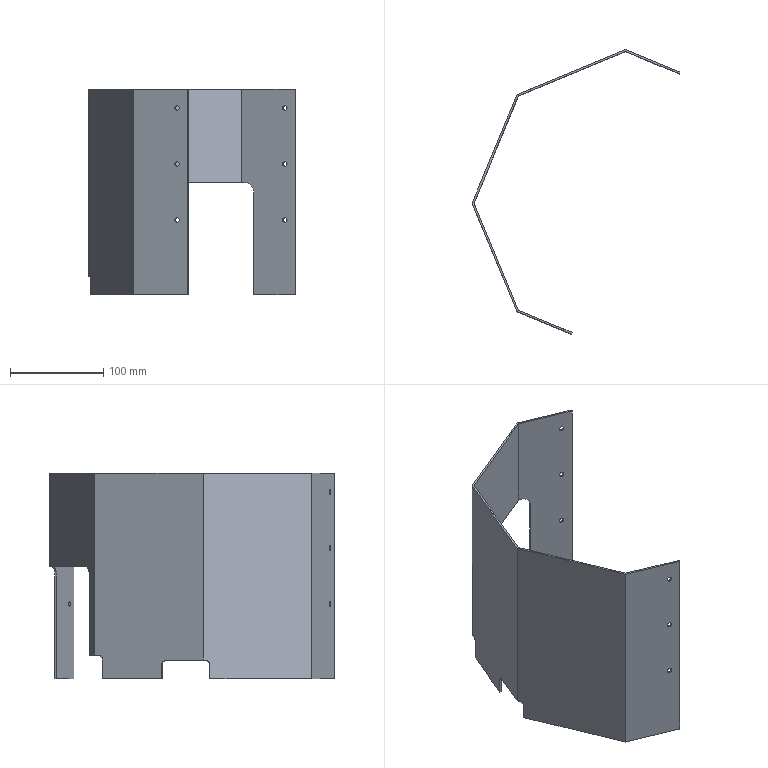Part | SolidWorks | features ICE 6, Fillet 3, Cut 2, Extrusion 1, RefAxis 1, Shell 1 | 1 solid | 41 faces | box 222.691 x 304.953 x 220 mm | volume 186706 mm3 | plane 24 | cylinder 17 | commonest cylinder face diameters 5 x12 10 x3 20 x2
STEP:
#1=CARTESIAN_POINT('',(-66.179,-134.946,80.));
#2=VERTEX_POINT('',#1);
#3=CARTESIAN_POINT('',(-70.799,-133.033,80.));
#4=VERTEX_POINT('',#3);
#5=CARTESIAN_POINT('',(-68.489,-133.99,80.));
#6=DIRECTION('',(0.3827,0.9239,0.));
#7=DIRECTION('',(-0.9239,0.3827,0.));
#8=AXIS2_PLACEMENT_3D('',#5,#6,#7);
#9=CIRCLE('',#8,2.5);
#10=EDGE_CURVE('',#2,#4,#9,.T.);
#11=ORIENTED_EDGE('',*,*,#10,.T.);
#12=CARTESIAN_POINT('',(-71.564,-134.881,80.));
#13=VERTEX_POINT('',#12);
#14=CARTESIAN_POINT('',(53.29,166.544,80.));
#15=DIRECTION('',(-0.3827,-0.9239,0.));
#16=VECTOR('',#15,1000.);
#17=LINE('',#14,#16);
#18=EDGE_CURVE('',#4,#13,#17,.T.);
#19=ORIENTED_EDGE('',*,*,#18,.T.);
#20=CARTESIAN_POINT('',(-66.945,-136.794,80.));
#21=VERTEX_POINT('',#20);
#22=CARTESIAN_POINT('',(-69.254,-135.837,80.));
#23=DIRECTION('',(-0.3827,-0.9239,0.));
#24=DIRECTION('',(0.9239,-0.3827,0.));
#25=AXIS2_PLACEMENT_3D('',#22,#23,#24);
#26=CIRCLE('',#25,2.5);
#27=EDGE_CURVE('',#13,#21,#26,.T.);
#28=ORIENTED_EDGE('',*,*,#27,.T.);
#29=CARTESIAN_POINT('',(57.91,164.631,80.));
#30=DIRECTION('',(-0.3827,-0.9239,0.));
#31=VECTOR('',#30,1000.);
#32=LINE('',#29,#31);
#33=EDGE_CURVE('',#2,#21,#32,.T.);
#34=ORIENTED_EDGE('',*,*,#33,.F.);
#35=EDGE_LOOP('',(#11,#19,#28,#34));
#36=FACE_OUTER_BOUND('',#35,.T.);
#37=CARTESIAN_POINT('',(55.6,165.587,80.));
#38=DIRECTION('',(-0.3827,-0.9239,0.));
#39=DIRECTION('',(0.9239,-0.3827,0.));
#40=AXIS2_PLACEMENT_3D('',#37,#38,#39);
#41=CYLINDRICAL_SURFACE('',#40,2.5);
#42=ADVANCED_FACE('',(#36),#41,.F.);
#43=CARTESIAN_POINT('',(44.772,145.979,80.));
#44=VERTEX_POINT('',#43);
#45=CARTESIAN_POINT('',(49.391,144.065,80.));
#46=VERTEX_POINT('',#45);
#47=CARTESIAN_POINT('',(47.081,145.022,80.));
#48=DIRECTION('',(-0.3827,-0.9239,0.));
#49=DIRECTION('',(0.9239,-0.3827,0.));
#50=AXIS2_PLACEMENT_3D('',#47,#48,#49);
#51=CIRCLE('',#50,2.5);
#52=EDGE_CURVE('',#44,#46,#51,.T.);
#53=ORIENTED_EDGE('',*,*,#52,.F.);
#54=CARTESIAN_POINT('',(44.006,144.131,80.));
#55=VERTEX_POINT('',#54);
#56=CARTESIAN_POINT('',(53.29,166.544,80.));
#57=DIRECTION('',(-0.3827,-0.9239,0.));
#58=VECTOR('',#57,1000.);
#59=LINE('',#56,#58);
#60=EDGE_CURVE('',#44,#55,#59,.T.);
#61=ORIENTED_EDGE('',*,*,#60,.T.);
#62=CARTESIAN_POINT('',(48.626,142.217,80.));
#63=VERTEX_POINT('',#62);
#64=CARTESIAN_POINT('',(46.316,143.174,80.));
#65=DIRECTION('',(-0.3827,-0.9239,0.));
#66=DIRECTION('',(0.9239,-0.3827,0.));
#67=AXIS2_PLACEMENT_3D('',#64,#65,#66);
#68=CIRCLE('',#67,2.5);
#69=EDGE_CURVE('',#55,#63,#68,.T.);
#70=ORIENTED_EDGE('',*,*,#69,.T.);
#71=CARTESIAN_POINT('',(57.91,164.631,80.));
#72=DIRECTION('',(-0.3827,-0.9239,0.));
#73=VECTOR('',#72,1000.);
#74=LINE('',#71,#73);
#75=EDGE_CURVE('',#46,#63,#74,.T.);
#76=ORIENTED_EDGE('',*,*,#75,.F.);
#77=EDGE_LOOP('',(#53,#61,#70,#76));
#78=FACE_OUTER_BOUND('',#77,.T.);
#79=CARTESIAN_POINT('',(55.6,165.587,80.));
#80=DIRECTION('',(-0.3827,-0.9239,0.));
#81=DIRECTION('',(0.9239,-0.3827,0.));
#82=AXIS2_PLACEMENT_3D('',#79,#80,#81);
#83=CYLINDRICAL_SURFACE('',#82,2.5);
#84=ADVANCED_FACE('',(#78),#83,.F.);
#85=CARTESIAN_POINT('',(-66.179,-134.946,140.));
#86=VERTEX_POINT('',#85);
#87=CARTESIAN_POINT('',(-70.799,-133.033,140.));
#88=VERTEX_POINT('',#87);
#89=CARTESIAN_POINT('',(-68.489,-133.99,140.));
#90=DIRECTION('',(0.3827,0.9239,0.));
#91=DIRECTION('',(-0.9239,0.3827,0.));
#92=AXIS2_PLACEMENT_3D('',#89,#90,#91);
#93=CIRCLE('',#92,2.5);
#94=EDGE_CURVE('',#86,#88,#93,.T.);
#95=ORIENTED_EDGE('',*,*,#94,.T.);
#96=CARTESIAN_POINT('',(-71.564,-134.881,140.));
#97=VERTEX_POINT('',#96);
#98=CARTESIAN_POINT('',(53.29,166.544,140.));
#99=DIRECTION('',(-0.3827,-0.9239,0.));
#100=VECTOR('',#99,1000.);
#101=LINE('',#98,#100);
#102=EDGE_CURVE('',#88,#97,#101,.T.);
#103=ORIENTED_EDGE('',*,*,#102,.T.);
#104=CARTESIAN_POINT('',(-66.945,-136.794,140.));
#105=VERTEX_POINT('',#104);
#106=CARTESIAN_POINT('',(-69.254,-135.837,140.));
#107=DIRECTION('',(-0.3827,-0.9239,0.));
#108=DIRECTION('',(0.9239,-0.3827,0.));
#109=AXIS2_PLACEMENT_3D('',#106,#107,#108);
#110=CIRCLE('',#109,2.5);
#111=EDGE_CURVE('',#97,#105,#110,.T.);
#112=ORIENTED_EDGE('',*,*,#111,.T.);
#113=CARTESIAN_POINT('',(57.91,164.631,140.));
#114=DIRECTION('',(-0.3827,-0.9239,0.));
#115=VECTOR('',#114,1000.);
#116=LINE('',#113,#115);
#117=EDGE_CURVE('',#86,#105,#116,.T.);
#118=ORIENTED_EDGE('',*,*,#117,.F.);
#119=EDGE_LOOP('',(#95,#103,#112,#118));
#120=FACE_OUTER_BOUND('',#119,.T.);
#121=CARTESIAN_POINT('',(55.6,165.587,140.));
#122=DIRECTION('',(-0.3827,-0.9239,0.));
#123=DIRECTION('',(0.9239,-0.3827,0.));
#124=AXIS2_PLACEMENT_3D('',#121,#122,#123);
#125=CYLINDRICAL_SURFACE('',#124,2.5);
#126=ADVANCED_FACE('',(#120),#125,.F.);
#127=CARTESIAN_POINT('',(44.772,145.979,140.));
#128=VERTEX_POINT('',#127);
#129=CARTESIAN_POINT('',(49.391,144.065,140.));
#130=VERTEX_POINT('',#129);
#131=CARTESIAN_POINT('',(47.081,145.022,140.));
#132=DIRECTION('',(-0.3827,-0.9239,0.));
#133=DIRECTION('',(0.9239,-0.3827,0.));
#134=AXIS2_PLACEMENT_3D('',#131,#132,#133);
#135=CIRCLE('',#134,2.5);
#136=EDGE_CURVE('',#128,#130,#135,.T.);
#137=ORIENTED_EDGE('',*,*,#136,.F.);
#138=CARTESIAN_POINT('',(44.006,144.131,140.));
#139=VERTEX_POINT('',#138);
#140=CARTESIAN_POINT('',(53.29,166.544,140.));
#141=DIRECTION('',(-0.3827,-0.9239,0.));
#142=VECTOR('',#141,1000.);
#143=LINE('',#140,#142);
#144=EDGE_CURVE('',#128,#139,#143,.T.);
#145=ORIENTED_EDGE('',*,*,#144,.T.);
#146=CARTESIAN_POINT('',(48.626,142.217,140.));
#147=VERTEX_POINT('',#146);
#148=CARTESIAN_POINT('',(46.316,143.174,140.));
#149=DIRECTION('',(-0.3827,-0.9239,0.));
#150=DIRECTION('',(0.9239,-0.3827,0.));
#151=AXIS2_PLACEMENT_3D('',#148,#149,#150);
#152=CIRCLE('',#151,2.5);
#153=EDGE_CURVE('',#139,#147,#152,.T.);
#154=ORIENTED_EDGE('',*,*,#153,.T.);
#155=CARTESIAN_POINT('',(57.91,164.631,140.));
#156=DIRECTION('',(-0.3827,-0.9239,0.));
#157=VECTOR('',#156,1000.);
#158=LINE('',#155,#157);
#159=EDGE_CURVE('',#130,#147,#158,.T.);
#160=ORIENTED_EDGE('',*,*,#159,.F.);
#161=EDGE_LOOP('',(#137,#145,#154,#160));
#162=FACE_OUTER_BOUND('',#161,.T.);
#163=CARTESIAN_POINT('',(55.6,165.587,140.));
#164=DIRECTION('',(-0.3827,-0.9239,0.));
#165=DIRECTION('',(0.9239,-0.3827,0.));
#166=AXIS2_PLACEMENT_3D('',#163,#164,#165);
#167=CYLINDRICAL_SURFACE('',#166,2.5);
#168=ADVANCED_FACE('',(#162),#167,.F.);
#169=CARTESIAN_POINT('',(-66.179,-134.946,200.));
#170=VERTEX_POINT('',#169);
#171=CARTESIAN_POINT('',(-70.799,-133.033,200.));
#172=VERTEX_POINT('',#171);
#173=CARTESIAN_POINT('',(-68.489,-133.99,200.));
#174=DIRECTION('',(0.3827,0.9239,0.));
#175=DIRECTION('',(-0.9239,0.3827,0.));
#176=AXIS2_PLACEMENT_3D('',#173,#174,#175);
#177=CIRCLE('',#176,2.5);
#178=EDGE_CURVE('',#170,#172,#177,.T.);
#179=ORIENTED_EDGE('',*,*,#178,.T.);
#180=CARTESIAN_POINT('',(-71.564,-134.881,200.));
#181=VERTEX_POINT('',#180);
#182=CARTESIAN_POINT('',(53.29,166.544,200.));
#183=DIRECTION('',(-0.3827,-0.9239,0.));
#184=VECTOR('',#183,1000.);
#185=LINE('',#182,#184);
#186=EDGE_CURVE('',#172,#181,#185,.T.);
#187=ORIENTED_EDGE('',*,*,#186,.T.);
#188=CARTESIAN_POINT('',(-66.945,-136.794,200.));
#189=VERTEX_POINT('',#188);
#190=CARTESIAN_POINT('',(-69.254,-135.837,200.));
#191=DIRECTION('',(-0.3827,-0.9239,0.));
#192=DIRECTION('',(0.9239,-0.3827,0.));
#193=AXIS2_PLACEMENT_3D('',#190,#191,#192);
#194=CIRCLE('',#193,2.5);
#195=EDGE_CURVE('',#181,#189,#194,.T.);
#196=ORIENTED_EDGE('',*,*,#195,.T.);
#197=CARTESIAN_POINT('',(57.91,164.631,200.));
#198=DIRECTION('',(-0.3827,-0.9239,0.));
#199=VECTOR('',#198,1000.);
#200=LINE('',#197,#199);
#201=EDGE_CURVE('',#170,#189,#200,.T.);
#202=ORIENTED_EDGE('',*,*,#201,.F.);
#203=EDGE_LOOP('',(#179,#187,#196,#202));
#204=FACE_OUTER_BOUND('',#203,.T.);
#205=CARTESIAN_POINT('',(55.6,165.587,200.));
#206=DIRECTION('',(-0.3827,-0.9239,0.));
#207=DIRECTION('',(0.9239,-0.3827,0.));
#208=AXIS2_PLACEMENT_3D('',#205,#206,#207);
#209=CYLINDRICAL_SURFACE('',#208,2.5);
#210=ADVANCED_FACE('',(#204),#209,.F.);
#211=CARTESIAN_POINT('',(44.772,145.979,200.));
#212=VERTEX_POINT('',#211);
#213=CARTESIAN_POINT('',(49.391,144.065,200.));
#214=VERTEX_POINT('',#213);
#215=CARTESIAN_POINT('',(47.081,145.022,200.));
#216=DIRECTION('',(-0.3827,-0.9239,0.));
#217=DIRECTION('',(0.9239,-0.3827,0.));
#218=AXIS2_PLACEMENT_3D('',#215,#216,#217);
#219=CIRCLE('',#218,2.5);
#220=EDGE_CURVE('',#212,#214,#219,.T.);
#221=ORIENTED_EDGE('',*,*,#220,.F.);
#222=CARTESIAN_POINT('',(44.006,144.131,200.));
#223=VERTEX_POINT('',#222);
#224=CARTESIAN_POINT('',(53.29,166.544,200.));
#225=DIRECTION('',(-0.3827,-0.9239,0.));
#226=VECTOR('',#225,1000.);
#227=LINE('',#224,#226);
#228=EDGE_CURVE('',#212,#223,#227,.T.);
#229=ORIENTED_EDGE('',*,*,#228,.T.);
#230=CARTESIAN_POINT('',(48.626,142.217,200.));
#231=VERTEX_POINT('',#230);
#232=CARTESIAN_POINT('',(46.316,143.174,200.));
#233=DIRECTION('',(-0.3827,-0.9239,0.));
#234=DIRECTION('',(0.9239,-0.3827,0.));
#235=AXIS2_PLACEMENT_3D('',#232,#233,#234);
#236=CIRCLE('',#235,2.5);
#237=EDGE_CURVE('',#223,#231,#236,.T.);
#238=ORIENTED_EDGE('',*,*,#237,.T.);
#239=CARTESIAN_POINT('',(57.91,164.631,200.));
#240=DIRECTION('',(-0.3827,-0.9239,0.));
#241=VECTOR('',#240,1000.);
#242=LINE('',#239,#241);
#243=EDGE_CURVE('',#214,#231,#242,.T.);
#244=ORIENTED_EDGE('',*,*,#243,.F.);
#245=EDGE_LOOP('',(#221,#229,#238,#244));
#246=FACE_OUTER_BOUND('',#245,.T.);
#247=CARTESIAN_POINT('',(55.6,165.587,200.));
#248=DIRECTION('',(-0.3827,-0.9239,0.));
#249=DIRECTION('',(0.9239,-0.3827,0.));
#250=AXIS2_PLACEMENT_3D('',#247,#248,#249);
#251=CYLINDRICAL_SURFACE('',#250,2.5);
#252=ADVANCED_FACE('',(#246),#251,.F.);
#253=CARTESIAN_POINT('',(-117.959,107.19,0.));
#254=VERTEX_POINT('',#253);
#255=CARTESIAN_POINT('',(-144.307,43.581,0.));
#256=VERTEX_POINT('',#255);
#257=CARTESIAN_POINT('',(-114.488,115.57,0.));
#258=DIRECTION('',(-0.3827,-0.9239,0.));
#259=VECTOR('',#258,1000.);
#260=LINE('',#257,#259);
#261=EDGE_CURVE('',#254,#256,#260,.T.);
#262=ORIENTED_EDGE('',*,*,#261,.T.);
#263=CARTESIAN_POINT('',(-146.155,44.346,0.));
#264=VERTEX_POINT('',#263);
#265=CARTESIAN_POINT('',(93.574,-54.953,0.));
#266=DIRECTION('',(-0.9239,0.3827,0.));
#267=VECTOR('',#266,1000.);
#268=LINE('',#265,#267);
#269=EDGE_CURVE('',#256,#264,#268,.T.);
#270=ORIENTED_EDGE('',*,*,#269,.T.);
#271=CARTESIAN_POINT('',(-119.807,107.955,0.));
#272=VERTEX_POINT('',#271);
#273=CARTESIAN_POINT('',(-116.336,116.336,0.));
#274=DIRECTION('',(-0.3827,-0.9239,0.));
#275=VECTOR('',#274,1000.);
#276=LINE('',#273,#275);
#277=EDGE_CURVE('',#272,#264,#276,.T.);
#278=ORIENTED_EDGE('',*,*,#277,.F.);
#279=CARTESIAN_POINT('',(-117.959,107.19,0.));
#280=DIRECTION('',(-0.9239,0.3827,0.));
#281=VECTOR('',#280,1000.);
#282=LINE('',#279,#281);
#283=EDGE_CURVE('',#254,#272,#282,.T.);
#284=ORIENTED_EDGE('',*,*,#283,.F.);
#285=EDGE_LOOP('',(#262,#270,#278,#284));
#286=FACE_OUTER_BOUND('',#285,.T.);
#287=CARTESIAN_POINT('',(0.,0.,0.));
#288=DIRECTION('',(0.,0.,1.));
#289=DIRECTION('',(1.,0.,0.));
#290=AXIS2_PLACEMENT_3D('',#287,#288,#289);
#291=PLANE('',#290);
#292=ADVANCED_FACE('',(#286),#291,.F.);
#293=CARTESIAN_POINT('',(57.403,138.582,0.));
#294=VERTEX_POINT('',#293);
#295=CARTESIAN_POINT('',(12.945,156.997,0.));
#296=VERTEX_POINT('',#295);
#297=CARTESIAN_POINT('',(115.57,114.488,0.));
#298=DIRECTION('',(-0.9239,0.3827,0.));
#299=VECTOR('',#298,1000.);
#300=LINE('',#297,#299);
#301=EDGE_CURVE('',#294,#296,#300,.T.);
#302=ORIENTED_EDGE('',*,*,#301,.T.);
#303=CARTESIAN_POINT('',(13.71,158.845,0.));
#304=VERTEX_POINT('',#303);
#305=CARTESIAN_POINT('',(12.945,156.997,0.));
#306=DIRECTION('',(-0.3827,-0.9239,0.));
#307=VECTOR('',#306,1000.);
#308=LINE('',#305,#307);
#309=EDGE_CURVE('',#304,#296,#308,.T.);
#310=ORIENTED_EDGE('',*,*,#309,.F.);
#311=CARTESIAN_POINT('',(58.168,140.43,0.));
#312=VERTEX_POINT('',#311);
#313=CARTESIAN_POINT('',(116.336,116.336,0.));
#314=DIRECTION('',(-0.9239,0.3827,0.));
#315=VECTOR('',#314,1000.);
#316=LINE('',#313,#315);
#317=EDGE_CURVE('',#312,#304,#316,.T.);
#318=ORIENTED_EDGE('',*,*,#317,.F.);
#319=CARTESIAN_POINT('',(75.617,182.555,0.));
#320=DIRECTION('',(-0.3827,-0.9239,0.));
#321=VECTOR('',#320,1000.);
#322=LINE('',#319,#321);
#323=EDGE_CURVE('',#312,#294,#322,.T.);
#324=ORIENTED_EDGE('',*,*,#323,.T.);
#325=EDGE_LOOP('',(#302,#310,#318,#324));
#326=FACE_OUTER_BOUND('',#325,.T.);
#327=CARTESIAN_POINT('',(0.,0.,0.));
#328=DIRECTION('',(0.,0.,1.));
#329=DIRECTION('',(1.,0.,0.));
#330=AXIS2_PLACEMENT_3D('',#327,#328,#329);
#331=PLANE('',#330);
#332=ADVANCED_FACE('',(#326),#331,.F.);
#333=CARTESIAN_POINT('',(-69.254,-135.837,80.));
#334=DIRECTION('',(-0.3827,-0.9239,0.));
#335=DIRECTION('',(0.9239,-0.3827,0.));
#336=AXIS2_PLACEMENT_3D('',#333,#334,#335);
#337=CIRCLE('',#336,2.5);
#338=EDGE_CURVE('',#21,#13,#337,.T.);
#339=ORIENTED_EDGE('',*,*,#338,.F.);
#340=ORIENTED_EDGE('',*,*,#27,.F.);
#341=EDGE_LOOP('',(#339,#340));
#342=FACE_BOUND('',#341,.T.);
#343=CARTESIAN_POINT('',(-69.254,-135.837,140.));
#344=DIRECTION('',(-0.3827,-0.9239,0.));
#345=DIRECTION('',(0.9239,-0.3827,0.));
#346=AXIS2_PLACEMENT_3D('',#343,#344,#345);
#347=CIRCLE('',#346,2.5);
#348=EDGE_CURVE('',#105,#97,#347,.T.);
#349=ORIENTED_EDGE('',*,*,#348,.F.);
#350=ORIENTED_EDGE('',*,*,#111,.F.);
#351=EDGE_LOOP('',(#349,#350));
#352=FACE_BOUND('',#351,.T.);
#353=CARTESIAN_POINT('',(-69.254,-135.837,200.));
#354=DIRECTION('',(-0.3827,-0.9239,0.));
#355=DIRECTION('',(0.9239,-0.3827,0.));
#356=AXIS2_PLACEMENT_3D('',#353,#354,#355);
#357=CIRCLE('',#356,2.5);
#358=EDGE_CURVE('',#189,#181,#357,.T.);
#359=ORIENTED_EDGE('',*,*,#358,.F.);
#360=ORIENTED_EDGE('',*,*,#195,.F.);
#361=EDGE_LOOP('',(#359,#360));
#362=FACE_BOUND('',#361,.T.);
#363=CARTESIAN_POINT('',(-116.336,-116.336,0.));
#364=VERTEX_POINT('',#363);
#365=CARTESIAN_POINT('',(-58.168,-140.43,0.));
#366=VERTEX_POINT('',#365);
#367=CARTESIAN_POINT('',(-116.336,-116.336,0.));
#368=DIRECTION('',(0.9239,-0.3827,0.));
#369=VECTOR('',#368,1000.);
#370=LINE('',#367,#369);
#371=EDGE_CURVE('',#364,#366,#370,.T.);
#372=ORIENTED_EDGE('',*,*,#371,.T.);
#373=CARTESIAN_POINT('',(-58.168,-140.43,220.));
#374=VERTEX_POINT('',#373);
#375=CARTESIAN_POINT('',(-58.168,-140.43,220.));
#376=DIRECTION('',(0.,0.,1.));
#377=VECTOR('',#376,1000.);
#378=LINE('',#375,#377);
#379=EDGE_CURVE('',#366,#374,#378,.T.);
#380=ORIENTED_EDGE('',*,*,#379,.T.);
#381=CARTESIAN_POINT('',(-116.336,-116.336,220.));
#382=VERTEX_POINT('',#381);
#383=CARTESIAN_POINT('',(-116.336,-116.336,220.));
#384=DIRECTION('',(0.9239,-0.3827,0.));
#385=VECTOR('',#384,1000.);
#386=LINE('',#383,#385);
#387=EDGE_CURVE('',#382,#374,#386,.T.);
#388=ORIENTED_EDGE('',*,*,#387,.F.);
#389=CARTESIAN_POINT('',(-116.336,-116.336,220.));
#390=DIRECTION('',(0.,0.,-1.));
#391=VECTOR('',#390,1000.);
#392=LINE('',#389,#391);
#393=EDGE_CURVE('',#382,#364,#392,.T.);
#394=ORIENTED_EDGE('',*,*,#393,.T.);
#395=EDGE_LOOP('',(#372,#380,#388,#394));
#396=FACE_OUTER_BOUND('',#395,.T.);
#397=CARTESIAN_POINT('',(-116.336,-116.336,220.));
#398=DIRECTION('',(0.3827,0.9239,0.));
#399=DIRECTION('',(-0.9239,0.3827,0.));
#400=AXIS2_PLACEMENT_3D('',#397,#398,#399);
#401=PLANE('',#400);
#402=ADVANCED_FACE('',(#342,#352,#362,#396),#401,.F.);
#403=CARTESIAN_POINT('',(47.081,145.022,80.));
#404=DIRECTION('',(-0.3827,-0.9239,0.));
#405=DIRECTION('',(0.9239,-0.3827,0.));
#406=AXIS2_PLACEMENT_3D('',#403,#404,#405);
#407=CIRCLE('',#406,2.5);
#408=EDGE_CURVE('',#46,#44,#407,.T.);
#409=ORIENTED_EDGE('',*,*,#408,.T.);
#410=ORIENTED_EDGE('',*,*,#52,.T.);
#411=EDGE_LOOP('',(#409,#410));
#412=FACE_BOUND('',#411,.T.);
#413=CARTESIAN_POINT('',(47.081,145.022,140.));
#414=DIRECTION('',(-0.3827,-0.9239,0.));
#415=DIRECTION('',(0.9239,-0.3827,0.));
#416=AXIS2_PLACEMENT_3D('',#413,#414,#415);
#417=CIRCLE('',#416,2.5);
#418=EDGE_CURVE('',#130,#128,#417,.T.);
#419=ORIENTED_EDGE('',*,*,#418,.T.);
#420=ORIENTED_EDGE('',*,*,#136,.T.);
#421=EDGE_LOOP('',(#419,#420));
#422=FACE_BOUND('',#421,.T.);
#423=CARTESIAN_POINT('',(47.081,145.022,200.));
#424=DIRECTION('',(-0.3827,-0.9239,0.));
#425=DIRECTION('',(0.9239,-0.3827,0.));
#426=AXIS2_PLACEMENT_3D('',#423,#424,#425);
#427=CIRCLE('',#426,2.5);
#428=EDGE_CURVE('',#214,#212,#427,.T.);
#429=ORIENTED_EDGE('',*,*,#428,.T.);
#430=ORIENTED_EDGE('',*,*,#220,.T.);
#431=EDGE_LOOP('',(#429,#430));
#432=FACE_BOUND('',#431,.T.);
#433=CARTESIAN_POINT('',(13.71,158.845,110.));
#434=VERTEX_POINT('',#433);
#435=CARTESIAN_POINT('',(13.71,158.845,123.2));
#436=DIRECTION('',(0.,0.,-1.));
#437=VECTOR('',#436,1000.);
#438=LINE('',#435,#437);
#439=EDGE_CURVE('',#434,#304,#438,.T.);
#440=ORIENTED_EDGE('',*,*,#439,.F.);
#441=CARTESIAN_POINT('',(4.471,162.672,120.));
#442=VERTEX_POINT('',#441);
#443=CARTESIAN_POINT('',(4.471,162.672,110.));
#444=DIRECTION('',(-0.3827,-0.9239,0.));
#445=DIRECTION('',(0.9239,-0.3827,0.));
#446=AXIS2_PLACEMENT_3D('',#443,#444,#445);
#447=CIRCLE('',#446,10.);
#448=EDGE_CURVE('',#434,#442,#447,.T.);
#449=ORIENTED_EDGE('',*,*,#448,.T.);
#450=CARTESIAN_POINT('',(0.,164.524,120.));
#451=VERTEX_POINT('',#450);
#452=CARTESIAN_POINT('',(116.336,116.336,120.));
#453=DIRECTION('',(-0.9239,0.3827,0.));
#454=VECTOR('',#453,1000.);
#455=LINE('',#452,#454);
#456=EDGE_CURVE('',#442,#451,#455,.T.);
#457=ORIENTED_EDGE('',*,*,#456,.T.);
#458=CARTESIAN_POINT('',(0.,164.524,220.));
#459=VERTEX_POINT('',#458);
#460=CARTESIAN_POINT('',(0.,164.524,220.));
#461=DIRECTION('',(0.,0.,-1.));
#462=VECTOR('',#461,1000.);
#463=LINE('',#460,#462);
#464=EDGE_CURVE('',#459,#451,#463,.T.);
#465=ORIENTED_EDGE('',*,*,#464,.F.);
#466=CARTESIAN_POINT('',(58.168,140.43,220.));
#467=VERTEX_POINT('',#466);
#468=CARTESIAN_POINT('',(116.336,116.336,220.));
#469=DIRECTION('',(-0.9239,0.3827,0.));
#470=VECTOR('',#469,1000.);
#471=LINE('',#468,#470);
#472=EDGE_CURVE('',#467,#459,#471,.T.);
#473=ORIENTED_EDGE('',*,*,#472,.F.);
#474=CARTESIAN_POINT('',(58.168,140.43,220.));
#475=DIRECTION('',(0.,0.,-1.));
#476=VECTOR('',#475,1000.);
#477=LINE('',#474,#476);
#478=EDGE_CURVE('',#467,#312,#477,.T.);
#479=ORIENTED_EDGE('',*,*,#478,.T.);
#480=ORIENTED_EDGE('',*,*,#317,.T.);
#481=EDGE_LOOP('',(#440,#449,#457,#465,#473,#479,#480));
#482=FACE_OUTER_BOUND('',#481,.T.);
#483=CARTESIAN_POINT('',(116.336,116.336,220.));
#484=DIRECTION('',(-0.3827,-0.9239,0.));
#485=DIRECTION('',(0.9239,-0.3827,0.));
#486=AXIS2_PLACEMENT_3D('',#483,#484,#485);
#487=PLANE('',#486);
#488=ADVANCED_FACE('',(#412,#422,#432,#482),#487,.F.);
#489=CARTESIAN_POINT('',(-102.478,122.076,25.));
#490=VERTEX_POINT('',#489);
#491=CARTESIAN_POINT('',(-102.478,122.076,110.));
#492=VERTEX_POINT('',#491);
#493=CARTESIAN_POINT('',(-102.478,122.076,0.));
#494=DIRECTION('',(0.,0.,1.));
#495=VECTOR('',#494,1000.);
#496=LINE('',#493,#495);
#497=EDGE_CURVE('',#490,#492,#496,.T.);
#498=ORIENTED_EDGE('',*,*,#497,.F.);
#499=CARTESIAN_POINT('',(-116.336,116.336,25.));
#500=VERTEX_POINT('',#499);
#501=CARTESIAN_POINT('',(-102.478,122.076,25.));
#502=DIRECTION('',(0.9239,0.3827,0.));
#503=VECTOR('',#502,1000.);
#504=LINE('',#501,#503);
#505=EDGE_CURVE('',#500,#490,#504,.T.);
#506=ORIENTED_EDGE('',*,*,#505,.F.);
#507=CARTESIAN_POINT('',(-116.336,116.336,220.));
#508=VERTEX_POINT('',#507);
#509=CARTESIAN_POINT('',(-116.336,116.336,220.));
#510=DIRECTION('',(0.,0.,-1.));
#511=VECTOR('',#510,1000.);
#512=LINE('',#509,#511);
#513=EDGE_CURVE('',#508,#500,#512,.T.);
#514=ORIENTED_EDGE('',*,*,#513,.F.);
#515=CARTESIAN_POINT('',(0.,164.524,220.));
#516=DIRECTION('',(-0.9239,-0.3827,0.));
#517=VECTOR('',#516,1000.);
#518=LINE('',#515,#517);
#519=EDGE_CURVE('',#459,#508,#518,.T.);
#520=ORIENTED_EDGE('',*,*,#519,.F.);
#521=ORIENTED_EDGE('',*,*,#464,.T.);
#522=CARTESIAN_POINT('',(-93.239,125.903,120.));
#523=VERTEX_POINT('',#522);
#524=CARTESIAN_POINT('',(8.388,167.998,120.));
#525=DIRECTION('',(0.9239,0.3827,0.));
#526=VECTOR('',#525,1000.);
#527=LINE('',#524,#526);
#528=EDGE_CURVE('',#523,#451,#527,.T.);
#529=ORIENTED_EDGE('',*,*,#528,.F.);
#530=CARTESIAN_POINT('',(-93.239,125.903,110.));
#531=DIRECTION('',(0.3827,-0.9239,0.));
#532=DIRECTION('',(0.9239,0.3827,0.));
#533=AXIS2_PLACEMENT_3D('',#530,#531,#532);
#534=CIRCLE('',#533,10.);
#535=EDGE_CURVE('',#523,#492,#534,.T.);
#536=ORIENTED_EDGE('',*,*,#535,.T.);
#537=EDGE_LOOP('',(#498,#506,#514,#520,#521,#529,#536));
#538=FACE_OUTER_BOUND('',#537,.T.);
#539=CARTESIAN_POINT('',(0.,164.524,220.));
#540=DIRECTION('',(0.3827,-0.9239,0.));
#541=DIRECTION('',(0.9239,0.3827,0.));
#542=AXIS2_PLACEMENT_3D('',#539,#540,#541);
#543=PLANE('',#542);
#544=ADVANCED_FACE('',(#538),#543,.F.);
#545=ORIENTED_EDGE('',*,*,#277,.T.);
#546=CARTESIAN_POINT('',(-146.155,44.346,15.));
#547=VERTEX_POINT('',#546);
#548=CARTESIAN_POINT('',(-146.155,44.346,0.));
#549=DIRECTION('',(0.,0.,-1.));
#550=VECTOR('',#549,1000.);
#551=LINE('',#548,#550);
#552=EDGE_CURVE('',#547,#264,#551,.T.);
#553=ORIENTED_EDGE('',*,*,#552,.F.);
#554=CARTESIAN_POINT('',(-148.068,39.727,20.));
#555=VERTEX_POINT('',#554);
#556=CARTESIAN_POINT('',(-148.068,39.727,15.));
#557=DIRECTION('',(0.9239,-0.3827,0.));
#558=DIRECTION('',(0.3827,0.9239,0.));
#559=AXIS2_PLACEMENT_3D('',#556,#557,#558);
#560=CIRCLE('',#559,5.);
#561=EDGE_CURVE('',#547,#555,#560,.T.);
#562=ORIENTED_EDGE('',*,*,#561,.T.);
#563=CARTESIAN_POINT('',(-164.524,0.,20.));
#564=VERTEX_POINT('',#563);
#565=CARTESIAN_POINT('',(-146.155,44.346,20.));
#566=DIRECTION('',(0.3827,0.9239,0.));
#567=VECTOR('',#566,1000.);
#568=LINE('',#565,#567);
#569=EDGE_CURVE('',#564,#555,#568,.T.);
#570=ORIENTED_EDGE('',*,*,#569,.F.);
#571=CARTESIAN_POINT('',(-164.524,0.,220.));
#572=VERTEX_POINT('',#571);
#573=CARTESIAN_POINT('',(-164.524,0.,220.));
#574=DIRECTION('',(0.,0.,-1.));
#575=VECTOR('',#574,1000.);
#576=LINE('',#573,#575);
#577=EDGE_CURVE('',#572,#564,#576,.T.);
#578=ORIENTED_EDGE('',*,*,#577,.F.);
#579=CARTESIAN_POINT('',(-116.336,116.336,220.));
#580=DIRECTION('',(-0.3827,-0.9239,0.));
#581=VECTOR('',#580,1000.);
#582=LINE('',#579,#581);
#583=EDGE_CURVE('',#508,#572,#582,.T.);
#584=ORIENTED_EDGE('',*,*,#583,.F.);
#585=ORIENTED_EDGE('',*,*,#513,.T.);
#586=CARTESIAN_POINT('',(-117.894,112.575,25.));
#587=VERTEX_POINT('',#586);
#588=CARTESIAN_POINT('',(-194.539,-72.463,25.));
#589=DIRECTION('',(0.3827,0.9239,0.));
#590=VECTOR('',#589,1000.);
#591=LINE('',#588,#590);
#592=EDGE_CURVE('',#587,#500,#591,.T.);
#593=ORIENTED_EDGE('',*,*,#592,.F.);
#594=CARTESIAN_POINT('',(-119.807,107.955,20.));
#595=VERTEX_POINT('',#594);
#596=CARTESIAN_POINT('',(-117.894,112.575,20.));
#597=DIRECTION('',(0.9239,-0.3827,0.));
#598=DIRECTION('',(0.3827,0.9239,0.));
#599=AXIS2_PLACEMENT_3D('',#596,#597,#598);
#600=CIRCLE('',#599,5.);
#601=EDGE_CURVE('',#587,#595,#600,.T.);
#602=ORIENTED_EDGE('',*,*,#601,.T.);
#603=CARTESIAN_POINT('',(-119.807,107.955,28.2));
#604=DIRECTION('',(0.,0.,-1.));
#605=VECTOR('',#604,1000.);
#606=LINE('',#603,#605);
#607=EDGE_CURVE('',#595,#272,#606,.T.);
#608=ORIENTED_EDGE('',*,*,#607,.T.);
#609=EDGE_LOOP('',(#545,#553,#562,#570,#578,#584,#585,#593,#602,#608));
#610=FACE_OUTER_BOUND('',#609,.T.);
#611=CARTESIAN_POINT('',(-116.336,116.336,220.));
#612=DIRECTION('',(0.9239,-0.3827,0.));
#613=DIRECTION('',(0.3827,0.9239,0.));
#614=AXIS2_PLACEMENT_3D('',#611,#612,#613);
#615=PLANE('',#614);
#616=ADVANCED_FACE('',(#610),#615,.F.);
#617=CARTESIAN_POINT('',(-163.507,-2.455,20.));
#618=VERTEX_POINT('',#617);
#619=CARTESIAN_POINT('',(-164.524,0.,20.));
#620=DIRECTION('',(0.3827,-0.9239,0.));
#621=VECTOR('',#620,1000.);
#622=LINE('',#619,#621);
#623=EDGE_CURVE('',#564,#618,#622,.T.);
#624=ORIENTED_EDGE('',*,*,#623,.T.);
#625=CARTESIAN_POINT('',(-161.593,-7.074,15.));
#626=VERTEX_POINT('',#625);
#627=CARTESIAN_POINT('',(-163.507,-2.455,15.));
#628=DIRECTION('',(0.9239,0.3827,0.));
#629=DIRECTION('',(-0.3827,0.9239,0.));
#630=AXIS2_PLACEMENT_3D('',#627,#628,#629);
#631=CIRCLE('',#630,5.);
#632=EDGE_CURVE('',#618,#626,#631,.T.);
#633=ORIENTED_EDGE('',*,*,#632,.T.);
#634=CARTESIAN_POINT('',(-161.593,-7.074,0.));
#635=VERTEX_POINT('',#634);
#636=CARTESIAN_POINT('',(-161.593,-7.074,23.2));
#637=DIRECTION('',(0.,0.,-1.));
#638=VECTOR('',#637,1000.);
#639=LINE('',#636,#638);
#640=EDGE_CURVE('',#626,#635,#639,.T.);
#641=ORIENTED_EDGE('',*,*,#640,.T.);
#642=CARTESIAN_POINT('',(-164.524,0.,0.));
#643=DIRECTION('',(0.3827,-0.9239,0.));
#644=VECTOR('',#643,1000.);
#645=LINE('',#642,#644);
#646=EDGE_CURVE('',#635,#364,#645,.T.);
#647=ORIENTED_EDGE('',*,*,#646,.T.);
#648=ORIENTED_EDGE('',*,*,#393,.F.);
#649=CARTESIAN_POINT('',(-164.524,0.,220.));
#650=DIRECTION('',(0.3827,-0.9239,0.));
#651=VECTOR('',#650,1000.);
#652=LINE('',#649,#651);
#653=EDGE_CURVE('',#572,#382,#652,.T.);
#654=ORIENTED_EDGE('',*,*,#653,.F.);
#655=ORIENTED_EDGE('',*,*,#577,.T.);
#656=EDGE_LOOP('',(#624,#633,#641,#647,#648,#654,#655));
#657=FACE_OUTER_BOUND('',#656,.T.);
#658=CARTESIAN_POINT('',(-164.524,0.,220.));
#659=DIRECTION('',(0.9239,0.3827,0.));
#660=DIRECTION('',(-0.3827,0.9239,0.));
#661=AXIS2_PLACEMENT_3D('',#658,#659,#660);
#662=PLANE('',#661);
#663=ADVANCED_FACE('',(#657),#662,.F.);
#664=CARTESIAN_POINT('',(57.403,138.582,220.));
#665=VERTEX_POINT('',#664);
#666=CARTESIAN_POINT('',(75.617,182.555,220.));
#667=DIRECTION('',(-0.3827,-0.9239,0.));
#668=VECTOR('',#667,1000.);
#669=LINE('',#666,#668);
#670=EDGE_CURVE('',#467,#665,#669,.T.);
#671=ORIENTED_EDGE('',*,*,#670,.F.);
#672=ORIENTED_EDGE('',*,*,#472,.T.);
#673=ORIENTED_EDGE('',*,*,#519,.T.);
#674=ORIENTED_EDGE('',*,*,#583,.T.);
#675=ORIENTED_EDGE('',*,*,#653,.T.);
#676=ORIENTED_EDGE('',*,*,#387,.T.);
#677=CARTESIAN_POINT('',(-57.403,-138.582,220.));
#678=VERTEX_POINT('',#677);
#679=CARTESIAN_POINT('',(75.617,182.555,220.));
#680=DIRECTION('',(-0.3827,-0.9239,0.));
#681=VECTOR('',#680,1000.);
#682=LINE('',#679,#681);
#683=EDGE_CURVE('',#678,#374,#682,.T.);
#684=ORIENTED_EDGE('',*,*,#683,.F.);
#685=CARTESIAN_POINT('',(-114.805,-114.805,220.));
#686=VERTEX_POINT('',#685);
#687=CARTESIAN_POINT('',(-115.57,-114.488,220.));
#688=DIRECTION('',(0.9239,-0.3827,0.));
#689=VECTOR('',#688,1000.);
#690=LINE('',#687,#689);
#691=EDGE_CURVE('',#686,#678,#690,.T.);
#692=ORIENTED_EDGE('',*,*,#691,.F.);
#693=CARTESIAN_POINT('',(-162.359,0.,220.));
#694=VERTEX_POINT('',#693);
#695=CARTESIAN_POINT('',(-162.676,0.7654,220.));
#696=DIRECTION('',(0.3827,-0.9239,0.));
#697=VECTOR('',#696,1000.);
#698=LINE('',#695,#697);
#699=EDGE_CURVE('',#694,#686,#698,.T.);
#700=ORIENTED_EDGE('',*,*,#699,.F.);
#701=CARTESIAN_POINT('',(-114.805,114.805,220.));
#702=VERTEX_POINT('',#701);
#703=CARTESIAN_POINT('',(-114.488,115.57,220.));
#704=DIRECTION('',(-0.3827,-0.9239,0.));
#705=VECTOR('',#704,1000.);
#706=LINE('',#703,#705);
#707=EDGE_CURVE('',#702,#694,#706,.T.);
#708=ORIENTED_EDGE('',*,*,#707,.F.);
#709=CARTESIAN_POINT('',(0.,162.359,220.));
#710=VERTEX_POINT('',#709);
#711=CARTESIAN_POINT('',(0.7654,162.676,220.));
#712=DIRECTION('',(-0.9239,-0.3827,0.));
#713=VECTOR('',#712,1000.);
#714=LINE('',#711,#713);
#715=EDGE_CURVE('',#710,#702,#714,.T.);
#716=ORIENTED_EDGE('',*,*,#715,.F.);
#717=CARTESIAN_POINT('',(115.57,114.488,220.));
#718=DIRECTION('',(-0.9239,0.3827,0.));
#719=VECTOR('',#718,1000.);
#720=LINE('',#717,#719);
#721=EDGE_CURVE('',#665,#710,#720,.T.);
#722=ORIENTED_EDGE('',*,*,#721,.F.);
#723=EDGE_LOOP('',(#671,#672,#673,#674,#675,#676,#684,#692,#700,#708,#716,#722));
#724=FACE_OUTER_BOUND('',#723,.T.);
#725=CARTESIAN_POINT('',(0.,0.,220.));
#726=DIRECTION('',(0.,0.,1.));
#727=DIRECTION('',(1.,0.,0.));
#728=AXIS2_PLACEMENT_3D('',#725,#726,#727);
#729=PLANE('',#728);
#730=ADVANCED_FACE('',(#724),#729,.T.);
#731=ORIENTED_EDGE('',*,*,#646,.F.);
#732=CARTESIAN_POINT('',(-159.746,-6.309,0.));
#733=VERTEX_POINT('',#732);
#734=CARTESIAN_POINT('',(-159.746,-6.309,0.));
#735=DIRECTION('',(-0.9239,-0.3827,0.));
#736=VECTOR('',#735,1000.);
#737=LINE('',#734,#736);
#738=EDGE_CURVE('',#733,#635,#737,.T.);
#739=ORIENTED_EDGE('',*,*,#738,.F.);
#740=CARTESIAN_POINT('',(-114.805,-114.805,0.));
#741=VERTEX_POINT('',#740);
#742=CARTESIAN_POINT('',(-162.676,0.7654,0.));
#743=DIRECTION('',(0.3827,-0.9239,0.));
#744=VECTOR('',#743,1000.);
#745=LINE('',#742,#744);
#746=EDGE_CURVE('',#733,#741,#745,.T.);
#747=ORIENTED_EDGE('',*,*,#746,.T.);
#748=CARTESIAN_POINT('',(-57.403,-138.582,0.));
#749=VERTEX_POINT('',#748);
#750=CARTESIAN_POINT('',(-115.57,-114.488,0.));
#751=DIRECTION('',(0.9239,-0.3827,0.));
#752=VECTOR('',#751,1000.);
#753=LINE('',#750,#752);
#754=EDGE_CURVE('',#741,#749,#753,.T.);
#755=ORIENTED_EDGE('',*,*,#754,.T.);
#756=CARTESIAN_POINT('',(75.617,182.555,0.));
#757=DIRECTION('',(-0.3827,-0.9239,0.));
#758=VECTOR('',#757,1000.);
#759=LINE('',#756,#758);
#760=EDGE_CURVE('',#749,#366,#759,.T.);
#761=ORIENTED_EDGE('',*,*,#760,.T.);
#762=ORIENTED_EDGE('',*,*,#371,.F.);
#763=EDGE_LOOP('',(#731,#739,#747,#755,#761,#762));
#764=FACE_OUTER_BOUND('',#763,.T.);
#765=CARTESIAN_POINT('',(0.,0.,0.));
#766=DIRECTION('',(0.,0.,1.));
#767=DIRECTION('',(1.,0.,0.));
#768=AXIS2_PLACEMENT_3D('',#765,#766,#767);
#769=PLANE('',#768);
#770=ADVANCED_FACE('',(#764),#769,.F.);
#771=ORIENTED_EDGE('',*,*,#10,.F.);
#772=CARTESIAN_POINT('',(-68.489,-133.99,80.));
#773=DIRECTION('',(0.3827,0.9239,0.));
#774=DIRECTION('',(-0.9239,0.3827,0.));
#775=AXIS2_PLACEMENT_3D('',#772,#773,#774);
#776=CIRCLE('',#775,2.5);
#777=EDGE_CURVE('',#4,#2,#776,.T.);
#778=ORIENTED_EDGE('',*,*,#777,.F.);
#779=EDGE_LOOP('',(#771,#778));
#780=FACE_BOUND('',#779,.T.);
#781=ORIENTED_EDGE('',*,*,#94,.F.);
#782=CARTESIAN_POINT('',(-68.489,-133.99,140.));
#783=DIRECTION('',(0.3827,0.9239,0.));
#784=DIRECTION('',(-0.9239,0.3827,0.));
#785=AXIS2_PLACEMENT_3D('',#782,#783,#784);
#786=CIRCLE('',#785,2.5);
#787=EDGE_CURVE('',#88,#86,#786,.T.);
#788=ORIENTED_EDGE('',*,*,#787,.F.);
#789=EDGE_LOOP('',(#781,#788));
#790=FACE_BOUND('',#789,.T.);
#791=ORIENTED_EDGE('',*,*,#178,.F.);
#792=CARTESIAN_POINT('',(-68.489,-133.99,200.));
#793=DIRECTION('',(0.3827,0.9239,0.));
#794=DIRECTION('',(-0.9239,0.3827,0.));
#795=AXIS2_PLACEMENT_3D('',#792,#793,#794);
#796=CIRCLE('',#795,2.5);
#797=EDGE_CURVE('',#172,#170,#796,.T.);
#798=ORIENTED_EDGE('',*,*,#797,.F.);
#799=EDGE_LOOP('',(#791,#798));
#800=FACE_BOUND('',#799,.T.);
#801=CARTESIAN_POINT('',(-57.403,-138.582,220.));
#802=DIRECTION('',(0.,0.,1.));
#803=VECTOR('',#802,1000.);
#804=LINE('',#801,#803);
#805=EDGE_CURVE('',#749,#678,#804,.T.);
#806=ORIENTED_EDGE('',*,*,#805,.F.);
#807=ORIENTED_EDGE('',*,*,#754,.F.);
#808=CARTESIAN_POINT('',(-114.805,-114.805,220.));
#809=DIRECTION('',(0.,0.,-1.));
#810=VECTOR('',#809,1000.);
#811=LINE('',#808,#810);
#812=EDGE_CURVE('',#686,#741,#811,.T.);
#813=ORIENTED_EDGE('',*,*,#812,.F.);
#814=ORIENTED_EDGE('',*,*,#691,.T.);
#815=EDGE_LOOP('',(#806,#807,#813,#814));
#816=FACE_OUTER_BOUND('',#815,.T.);
#817=CARTESIAN_POINT('',(-115.57,-114.488,220.));
#818=DIRECTION('',(0.3827,0.9239,0.));
#819=DIRECTION('',(-0.9239,0.3827,0.));
#820=AXIS2_PLACEMENT_3D('',#817,#818,#819);
#821=PLANE('',#820);
#822=ADVANCED_FACE('',(#780,#790,#800,#816),#821,.T.);
#823=CARTESIAN_POINT('',(12.945,156.997,110.));
#824=VERTEX_POINT('',#823);
#825=CARTESIAN_POINT('',(12.945,156.997,220.));
#826=DIRECTION('',(0.,0.,1.));
#827=VECTOR('',#826,1000.);
#828=LINE('',#825,#827);
#829=EDGE_CURVE('',#296,#824,#828,.T.);
#830=ORIENTED_EDGE('',*,*,#829,.F.);
#831=ORIENTED_EDGE('',*,*,#301,.F.);
#832=CARTESIAN_POINT('',(57.403,138.582,220.));
#833=DIRECTION('',(0.,0.,-1.));
#834=VECTOR('',#833,1000.);
#835=LINE('',#832,#834);
#836=EDGE_CURVE('',#665,#294,#835,.T.);
#837=ORIENTED_EDGE('',*,*,#836,.F.);
#838=ORIENTED_EDGE('',*,*,#721,.T.);
#839=CARTESIAN_POINT('',(0.,162.359,120.));
#840=VERTEX_POINT('',#839);
#841=CARTESIAN_POINT('',(0.,162.359,220.));
#842=DIRECTION('',(0.,0.,-1.));
#843=VECTOR('',#842,1000.);
#844=LINE('',#841,#843);
#845=EDGE_CURVE('',#710,#840,#844,.T.);
#846=ORIENTED_EDGE('',*,*,#845,.T.);
#847=CARTESIAN_POINT('',(3.706,160.824,120.));
#848=VERTEX_POINT('',#847);
#849=CARTESIAN_POINT('',(115.57,114.488,120.));
#850=DIRECTION('',(-0.9239,0.3827,0.));
#851=VECTOR('',#850,1000.);
#852=LINE('',#849,#851);
#853=EDGE_CURVE('',#848,#840,#852,.T.);
#854=ORIENTED_EDGE('',*,*,#853,.F.);
#855=CARTESIAN_POINT('',(3.706,160.824,110.));
#856=DIRECTION('',(0.3827,0.9239,0.));
#857=DIRECTION('',(0.9239,-0.3827,0.));
#858=AXIS2_PLACEMENT_3D('',#855,#856,#857);
#859=CIRCLE('',#858,10.);
#860=EDGE_CURVE('',#848,#824,#859,.T.);
#861=ORIENTED_EDGE('',*,*,#860,.T.);
#862=EDGE_LOOP('',(#830,#831,#837,#838,#846,#854,#861));
#863=FACE_OUTER_BOUND('',#862,.T.);
#864=CARTESIAN_POINT('',(46.316,143.174,80.));
#865=DIRECTION('',(-0.3827,-0.9239,0.));
#866=DIRECTION('',(0.9239,-0.3827,0.));
#867=AXIS2_PLACEMENT_3D('',#864,#865,#866);
#868=CIRCLE('',#867,2.5);
#869=EDGE_CURVE('',#63,#55,#868,.T.);
#870=ORIENTED_EDGE('',*,*,#869,.F.);
#871=ORIENTED_EDGE('',*,*,#69,.F.);
#872=EDGE_LOOP('',(#870,#871));
#873=FACE_BOUND('',#872,.T.);
#874=CARTESIAN_POINT('',(46.316,143.174,140.));
#875=DIRECTION('',(-0.3827,-0.9239,0.));
#876=DIRECTION('',(0.9239,-0.3827,0.));
#877=AXIS2_PLACEMENT_3D('',#874,#875,#876);
#878=CIRCLE('',#877,2.5);
#879=EDGE_CURVE('',#147,#139,#878,.T.);
#880=ORIENTED_EDGE('',*,*,#879,.F.);
#881=ORIENTED_EDGE('',*,*,#153,.F.);
#882=EDGE_LOOP('',(#880,#881));
#883=FACE_BOUND('',#882,.T.);
#884=CARTESIAN_POINT('',(46.316,143.174,200.));
#885=DIRECTION('',(-0.3827,-0.9239,0.));
#886=DIRECTION('',(0.9239,-0.3827,0.));
#887=AXIS2_PLACEMENT_3D('',#884,#885,#886);
#888=CIRCLE('',#887,2.5);
#889=EDGE_CURVE('',#231,#223,#888,.T.);
#890=ORIENTED_EDGE('',*,*,#889,.F.);
#891=ORIENTED_EDGE('',*,*,#237,.F.);
#892=EDGE_LOOP('',(#890,#891));
#893=FACE_BOUND('',#892,.T.);
#894=CARTESIAN_POINT('',(115.57,114.488,220.));
#895=DIRECTION('',(-0.3827,-0.9239,0.));
#896=DIRECTION('',(0.9239,-0.3827,0.));
#897=AXIS2_PLACEMENT_3D('',#894,#895,#896);
#898=PLANE('',#897);
#899=ADVANCED_FACE('',(#863,#873,#883,#893),#898,.T.);
#900=CARTESIAN_POINT('',(-114.805,114.805,25.));
#901=VERTEX_POINT('',#900);
#902=CARTESIAN_POINT('',(-101.712,120.228,25.));
#903=VERTEX_POINT('',#902);
#904=CARTESIAN_POINT('',(-101.712,120.228,25.));
#905=DIRECTION('',(0.9239,0.3827,0.));
#906=VECTOR('',#905,1000.);
#907=LINE('',#904,#906);
#908=EDGE_CURVE('',#901,#903,#907,.T.);
#909=ORIENTED_EDGE('',*,*,#908,.T.);
#910=CARTESIAN_POINT('',(-101.712,120.228,110.));
#911=VERTEX_POINT('',#910);
#912=CARTESIAN_POINT('',(-101.712,120.228,220.));
#913=DIRECTION('',(0.,0.,-1.));
#914=VECTOR('',#913,1000.);
#915=LINE('',#912,#914);
#916=EDGE_CURVE('',#911,#903,#915,.T.);
#917=ORIENTED_EDGE('',*,*,#916,.F.);
#918=CARTESIAN_POINT('',(-92.473,124.055,120.));
#919=VERTEX_POINT('',#918);
#920=CARTESIAN_POINT('',(-92.473,124.055,110.));
#921=DIRECTION('',(-0.3827,0.9239,0.));
#922=DIRECTION('',(0.9239,0.3827,0.));
#923=AXIS2_PLACEMENT_3D('',#920,#921,#922);
#924=CIRCLE('',#923,10.);
#925=EDGE_CURVE('',#911,#919,#924,.T.);
#926=ORIENTED_EDGE('',*,*,#925,.T.);
#927=CARTESIAN_POINT('',(0.7654,162.676,120.));
#928=DIRECTION('',(-0.9239,-0.3827,0.));
#929=VECTOR('',#928,1000.);
#930=LINE('',#927,#929);
#931=EDGE_CURVE('',#840,#919,#930,.T.);
#932=ORIENTED_EDGE('',*,*,#931,.F.);
#933=ORIENTED_EDGE('',*,*,#845,.F.);
#934=ORIENTED_EDGE('',*,*,#715,.T.);
#935=CARTESIAN_POINT('',(-114.805,114.805,220.));
#936=DIRECTION('',(0.,0.,-1.));
#937=VECTOR('',#936,1000.);
#938=LINE('',#935,#937);
#939=EDGE_CURVE('',#702,#901,#938,.T.);
#940=ORIENTED_EDGE('',*,*,#939,.T.);
#941=EDGE_LOOP('',(#909,#917,#926,#932,#933,#934,#940));
#942=FACE_OUTER_BOUND('',#941,.T.);
#943=CARTESIAN_POINT('',(0.7654,162.676,220.));
#944=DIRECTION('',(0.3827,-0.9239,0.));
#945=DIRECTION('',(0.9239,0.3827,0.));
#946=AXIS2_PLACEMENT_3D('',#943,#944,#945);
#947=PLANE('',#946);
#948=ADVANCED_FACE('',(#942),#947,.T.);
#949=CARTESIAN_POINT('',(-144.307,43.581,15.));
#950=VERTEX_POINT('',#949);
#951=CARTESIAN_POINT('',(-144.307,43.581,220.));
#952=DIRECTION('',(0.,0.,1.));
#953=VECTOR('',#952,1000.);
#954=LINE('',#951,#953);
#955=EDGE_CURVE('',#256,#950,#954,.T.);
#956=ORIENTED_EDGE('',*,*,#955,.F.);
#957=ORIENTED_EDGE('',*,*,#261,.F.);
#958=CARTESIAN_POINT('',(-117.959,107.19,20.));
#959=VERTEX_POINT('',#958);
#960=CARTESIAN_POINT('',(-117.959,107.19,0.));
#961=DIRECTION('',(0.,0.,1.));
#962=VECTOR('',#961,1000.);
#963=LINE('',#960,#962);
#964=EDGE_CURVE('',#254,#959,#963,.T.);
#965=ORIENTED_EDGE('',*,*,#964,.T.);
#966=CARTESIAN_POINT('',(-116.046,111.809,25.));
#967=VERTEX_POINT('',#966);
#968=CARTESIAN_POINT('',(-116.046,111.809,20.));
#969=DIRECTION('',(-0.9239,0.3827,0.));
#970=DIRECTION('',(0.3827,0.9239,0.));
#971=AXIS2_PLACEMENT_3D('',#968,#969,#970);
#972=CIRCLE('',#971,5.);
#973=EDGE_CURVE('',#959,#967,#972,.T.);
#974=ORIENTED_EDGE('',*,*,#973,.T.);
#975=CARTESIAN_POINT('',(-192.691,-73.229,25.));
#976=DIRECTION('',(0.3827,0.9239,0.));
#977=VECTOR('',#976,1000.);
#978=LINE('',#975,#977);
#979=EDGE_CURVE('',#967,#901,#978,.T.);
#980=ORIENTED_EDGE('',*,*,#979,.T.);
#981=ORIENTED_EDGE('',*,*,#939,.F.);
#982=ORIENTED_EDGE('',*,*,#707,.T.);
#983=CARTESIAN_POINT('',(-162.359,0.,20.));
#984=VERTEX_POINT('',#983);
#985=CARTESIAN_POINT('',(-162.359,0.,220.));
#986=DIRECTION('',(0.,0.,-1.));
#987=VECTOR('',#986,1000.);
#988=LINE('',#985,#987);
#989=EDGE_CURVE('',#694,#984,#988,.T.);
#990=ORIENTED_EDGE('',*,*,#989,.T.);
#991=CARTESIAN_POINT('',(-146.22,38.961,20.));
#992=VERTEX_POINT('',#991);
#993=CARTESIAN_POINT('',(-114.488,115.57,20.));
#994=DIRECTION('',(-0.3827,-0.9239,0.));
#995=VECTOR('',#994,1000.);
#996=LINE('',#993,#995);
#997=EDGE_CURVE('',#992,#984,#996,.T.);
#998=ORIENTED_EDGE('',*,*,#997,.F.);
#999=CARTESIAN_POINT('',(-146.22,38.961,15.));
#1000=DIRECTION('',(-0.9239,0.3827,0.));
#1001=DIRECTION('',(0.3827,0.9239,0.));
#1002=AXIS2_PLACEMENT_3D('',#999,#1000,#1001);
#1003=CIRCLE('',#1002,5.);
#1004=EDGE_CURVE('',#992,#950,#1003,.T.);
#1005=ORIENTED_EDGE('',*,*,#1004,.T.);
#1006=EDGE_LOOP('',(#956,#957,#965,#974,#980,#981,#982,#990,#998,#1005));
#1007=FACE_OUTER_BOUND('',#1006,.T.);
#1008=CARTESIAN_POINT('',(-114.488,115.57,220.));
#1009=DIRECTION('',(0.9239,-0.3827,0.));
#1010=DIRECTION('',(0.3827,0.9239,0.));
#1011=AXIS2_PLACEMENT_3D('',#1008,#1009,#1010);
#1012=PLANE('',#1011);
#1013=ADVANCED_FACE('',(#1007),#1012,.T.);
#1014=CARTESIAN_POINT('',(-161.659,-1.689,20.));
#1015=VERTEX_POINT('',#1014);
#1016=CARTESIAN_POINT('',(-162.676,0.7654,20.));
#1017=DIRECTION('',(0.3827,-0.9239,0.));
#1018=VECTOR('',#1017,1000.);
#1019=LINE('',#1016,#1018);
#1020=EDGE_CURVE('',#984,#1015,#1019,.T.);
#1021=ORIENTED_EDGE('',*,*,#1020,.F.);
#1022=ORIENTED_EDGE('',*,*,#989,.F.);
#1023=ORIENTED_EDGE('',*,*,#699,.T.);
#1024=ORIENTED_EDGE('',*,*,#812,.T.);
#1025=ORIENTED_EDGE('',*,*,#746,.F.);
#1026=CARTESIAN_POINT('',(-159.746,-6.309,15.));
#1027=VERTEX_POINT('',#1026);
#1028=CARTESIAN_POINT('',(-159.746,-6.309,220.));
#1029=DIRECTION('',(0.,0.,-1.));
#1030=VECTOR('',#1029,1000.);
#1031=LINE('',#1028,#1030);
#1032=EDGE_CURVE('',#1027,#733,#1031,.T.);
#1033=ORIENTED_EDGE('',*,*,#1032,.F.);
#1034=CARTESIAN_POINT('',(-161.659,-1.689,15.));
#1035=DIRECTION('',(-0.9239,-0.3827,0.));
#1036=DIRECTION('',(-0.3827,0.9239,0.));
#1037=AXIS2_PLACEMENT_3D('',#1034,#1035,#1036);
#1038=CIRCLE('',#1037,5.);
#1039=EDGE_CURVE('',#1027,#1015,#1038,.T.);
#1040=ORIENTED_EDGE('',*,*,#1039,.T.);
#1041=EDGE_LOOP('',(#1021,#1022,#1023,#1024,#1025,#1033,#1040));
#1042=FACE_OUTER_BOUND('',#1041,.T.);
#1043=CARTESIAN_POINT('',(-162.676,0.7654,220.));
#1044=DIRECTION('',(0.9239,0.3827,0.));
#1045=DIRECTION('',(-0.3827,0.9239,0.));
#1046=AXIS2_PLACEMENT_3D('',#1043,#1044,#1045);
#1047=PLANE('',#1046);
#1048=ADVANCED_FACE('',(#1042),#1047,.T.);
#1049=ORIENTED_EDGE('',*,*,#670,.T.);
#1050=ORIENTED_EDGE('',*,*,#836,.T.);
#1051=ORIENTED_EDGE('',*,*,#323,.F.);
#1052=ORIENTED_EDGE('',*,*,#478,.F.);
#1053=EDGE_LOOP('',(#1049,#1050,#1051,#1052));
#1054=FACE_OUTER_BOUND('',#1053,.T.);
#1055=CARTESIAN_POINT('',(75.617,182.555,0.));
#1056=DIRECTION('',(-0.9239,0.3827,0.));
#1057=DIRECTION('',(-0.3827,-0.9239,0.));
#1058=AXIS2_PLACEMENT_3D('',#1055,#1056,#1057);
#1059=PLANE('',#1058);
#1060=ADVANCED_FACE('',(#1054),#1059,.F.);
#1061=ORIENTED_EDGE('',*,*,#760,.F.);
#1062=ORIENTED_EDGE('',*,*,#805,.T.);
#1063=ORIENTED_EDGE('',*,*,#683,.T.);
#1064=ORIENTED_EDGE('',*,*,#379,.F.);
#1065=EDGE_LOOP('',(#1061,#1062,#1063,#1064));
#1066=FACE_OUTER_BOUND('',#1065,.T.);
#1067=CARTESIAN_POINT('',(75.617,182.555,0.));
#1068=DIRECTION('',(-0.9239,0.3827,0.));
#1069=DIRECTION('',(-0.3827,-0.9239,0.));
#1070=AXIS2_PLACEMENT_3D('',#1067,#1068,#1069);
#1071=PLANE('',#1070);
#1072=ADVANCED_FACE('',(#1066),#1071,.F.);
#1073=ORIENTED_EDGE('',*,*,#228,.F.);
#1074=ORIENTED_EDGE('',*,*,#428,.F.);
#1075=ORIENTED_EDGE('',*,*,#243,.T.);
#1076=ORIENTED_EDGE('',*,*,#889,.T.);
#1077=EDGE_LOOP('',(#1073,#1074,#1075,#1076));
#1078=FACE_OUTER_BOUND('',#1077,.T.);
#1079=CARTESIAN_POINT('',(55.6,165.587,200.));
#1080=DIRECTION('',(-0.3827,-0.9239,0.));
#1081=DIRECTION('',(0.9239,-0.3827,0.));
#1082=AXIS2_PLACEMENT_3D('',#1079,#1080,#1081);
#1083=CYLINDRICAL_SURFACE('',#1082,2.5);
#1084=ADVANCED_FACE('',(#1078),#1083,.F.);
#1085=ORIENTED_EDGE('',*,*,#186,.F.);
#1086=ORIENTED_EDGE('',*,*,#797,.T.);
#1087=ORIENTED_EDGE('',*,*,#201,.T.);
#1088=ORIENTED_EDGE('',*,*,#358,.T.);
#1089=EDGE_LOOP('',(#1085,#1086,#1087,#1088));
#1090=FACE_OUTER_BOUND('',#1089,.T.);
#1091=CARTESIAN_POINT('',(55.6,165.587,200.));
#1092=DIRECTION('',(-0.3827,-0.9239,0.));
#1093=DIRECTION('',(0.9239,-0.3827,0.));
#1094=AXIS2_PLACEMENT_3D('',#1091,#1092,#1093);
#1095=CYLINDRICAL_SURFACE('',#1094,2.5);
#1096=ADVANCED_FACE('',(#1090),#1095,.F.);
#1097=ORIENTED_EDGE('',*,*,#144,.F.);
#1098=ORIENTED_EDGE('',*,*,#418,.F.);
#1099=ORIENTED_EDGE('',*,*,#159,.T.);
#1100=ORIENTED_EDGE('',*,*,#879,.T.);
#1101=EDGE_LOOP('',(#1097,#1098,#1099,#1100));
#1102=FACE_OUTER_BOUND('',#1101,.T.);
#1103=CARTESIAN_POINT('',(55.6,165.587,140.));
#1104=DIRECTION('',(-0.3827,-0.9239,0.));
#1105=DIRECTION('',(0.9239,-0.3827,0.));
#1106=AXIS2_PLACEMENT_3D('',#1103,#1104,#1105);
#1107=CYLINDRICAL_SURFACE('',#1106,2.5);
#1108=ADVANCED_FACE('',(#1102),#1107,.F.);
#1109=ORIENTED_EDGE('',*,*,#102,.F.);
#1110=ORIENTED_EDGE('',*,*,#787,.T.);
#1111=ORIENTED_EDGE('',*,*,#117,.T.);
#1112=ORIENTED_EDGE('',*,*,#348,.T.);
#1113=EDGE_LOOP('',(#1109,#1110,#1111,#1112));
#1114=FACE_OUTER_BOUND('',#1113,.T.);
#1115=CARTESIAN_POINT('',(55.6,165.587,140.));
#1116=DIRECTION('',(-0.3827,-0.9239,0.));
#1117=DIRECTION('',(0.9239,-0.3827,0.));
#1118=AXIS2_PLACEMENT_3D('',#1115,#1116,#1117);
#1119=CYLINDRICAL_SURFACE('',#1118,2.5);
#1120=ADVANCED_FACE('',(#1114),#1119,.F.);
#1121=ORIENTED_EDGE('',*,*,#60,.F.);
#1122=ORIENTED_EDGE('',*,*,#408,.F.);
#1123=ORIENTED_EDGE('',*,*,#75,.T.);
#1124=ORIENTED_EDGE('',*,*,#869,.T.);
#1125=EDGE_LOOP('',(#1121,#1122,#1123,#1124));
#1126=FACE_OUTER_BOUND('',#1125,.T.);
#1127=CARTESIAN_POINT('',(55.6,165.587,80.));
#1128=DIRECTION('',(-0.3827,-0.9239,0.));
#1129=DIRECTION('',(0.9239,-0.3827,0.));
#1130=AXIS2_PLACEMENT_3D('',#1127,#1128,#1129);
#1131=CYLINDRICAL_SURFACE('',#1130,2.5);
#1132=ADVANCED_FACE('',(#1126),#1131,.F.);
#1133=ORIENTED_EDGE('',*,*,#18,.F.);
#1134=ORIENTED_EDGE('',*,*,#777,.T.);
#1135=ORIENTED_EDGE('',*,*,#33,.T.);
#1136=ORIENTED_EDGE('',*,*,#338,.T.);
#1137=EDGE_LOOP('',(#1133,#1134,#1135,#1136));
#1138=FACE_OUTER_BOUND('',#1137,.T.);
#1139=CARTESIAN_POINT('',(55.6,165.587,80.));
#1140=DIRECTION('',(-0.3827,-0.9239,0.));
#1141=DIRECTION('',(0.9239,-0.3827,0.));
#1142=AXIS2_PLACEMENT_3D('',#1139,#1140,#1141);
#1143=CYLINDRICAL_SURFACE('',#1142,2.5);
#1144=ADVANCED_FACE('',(#1138),#1143,.F.);
#1145=ORIENTED_EDGE('',*,*,#931,.T.);
#1146=CARTESIAN_POINT('',(-93.239,125.903,120.));
#1147=DIRECTION('',(-0.3827,0.9239,0.));
#1148=VECTOR('',#1147,1000.);
#1149=LINE('',#1146,#1148);
#1150=EDGE_CURVE('',#919,#523,#1149,.T.);
#1151=ORIENTED_EDGE('',*,*,#1150,.T.);
#1152=ORIENTED_EDGE('',*,*,#528,.T.);
#1153=ORIENTED_EDGE('',*,*,#456,.F.);
#1154=CARTESIAN_POINT('',(3.706,160.824,120.));
#1155=DIRECTION('',(-0.3827,-0.9239,0.));
#1156=VECTOR('',#1155,1000.);
#1157=LINE('',#1154,#1156);
#1158=EDGE_CURVE('',#442,#848,#1157,.T.);
#1159=ORIENTED_EDGE('',*,*,#1158,.T.);
#1160=ORIENTED_EDGE('',*,*,#853,.T.);
#1161=EDGE_LOOP('',(#1145,#1151,#1152,#1153,#1159,#1160));
#1162=FACE_OUTER_BOUND('',#1161,.T.);
#1163=CARTESIAN_POINT('',(124.724,-112.861,120.));
#1164=DIRECTION('',(0.,0.,1.));
#1165=DIRECTION('',(1.,0.,0.));
#1166=AXIS2_PLACEMENT_3D('',#1163,#1164,#1165);
#1167=PLANE('',#1166);
#1168=ADVANCED_FACE('',(#1162),#1167,.F.);
#1169=ORIENTED_EDGE('',*,*,#916,.T.);
#1170=CARTESIAN_POINT('',(13.859,-158.785,25.));
#1171=DIRECTION('',(-0.3827,0.9239,0.));
#1172=VECTOR('',#1171,1000.);
#1173=LINE('',#1170,#1172);
#1174=EDGE_CURVE('',#903,#490,#1173,.T.);
#1175=ORIENTED_EDGE('',*,*,#1174,.T.);
#1176=ORIENTED_EDGE('',*,*,#497,.T.);
#1177=CARTESIAN_POINT('',(-101.712,120.228,110.));
#1178=DIRECTION('',(0.3827,-0.9239,0.));
#1179=VECTOR('',#1178,1000.);
#1180=LINE('',#1177,#1179);
#1181=EDGE_CURVE('',#492,#911,#1180,.T.);
#1182=ORIENTED_EDGE('',*,*,#1181,.T.);
#1183=EDGE_LOOP('',(#1169,#1175,#1176,#1182));
#1184=FACE_OUTER_BOUND('',#1183,.T.);
#1185=CARTESIAN_POINT('',(13.858,-158.783,0.));
#1186=DIRECTION('',(-0.9239,-0.3827,0.));
#1187=DIRECTION('',(0.3827,-0.9239,0.));
#1188=AXIS2_PLACEMENT_3D('',#1185,#1186,#1187);
#1189=PLANE('',#1188);
#1190=ADVANCED_FACE('',(#1184),#1189,.F.);
#1191=ORIENTED_EDGE('',*,*,#829,.T.);
#1192=CARTESIAN_POINT('',(13.71,158.845,110.));
#1193=DIRECTION('',(0.3827,0.9239,0.));
#1194=VECTOR('',#1193,1000.);
#1195=LINE('',#1192,#1194);
#1196=EDGE_CURVE('',#824,#434,#1195,.T.);
#1197=ORIENTED_EDGE('',*,*,#1196,.T.);
#1198=ORIENTED_EDGE('',*,*,#439,.T.);
#1199=ORIENTED_EDGE('',*,*,#309,.T.);
#1200=EDGE_LOOP('',(#1191,#1197,#1198,#1199));
#1201=FACE_OUTER_BOUND('',#1200,.T.);
#1202=CARTESIAN_POINT('',(12.945,156.997,123.2));
#1203=DIRECTION('',(0.9239,-0.3827,0.));
#1204=DIRECTION('',(0.3827,0.9239,0.));
#1205=AXIS2_PLACEMENT_3D('',#1202,#1203,#1204);
#1206=PLANE('',#1205);
#1207=ADVANCED_FACE('',(#1201),#1206,.F.);
#1208=ORIENTED_EDGE('',*,*,#925,.F.);
#1209=ORIENTED_EDGE('',*,*,#1181,.F.);
#1210=ORIENTED_EDGE('',*,*,#535,.F.);
#1211=ORIENTED_EDGE('',*,*,#1150,.F.);
#1212=EDGE_LOOP('',(#1208,#1209,#1210,#1211));
#1213=FACE_OUTER_BOUND('',#1212,.T.);
#1214=CARTESIAN_POINT('',(23.097,-154.957,110.));
#1215=DIRECTION('',(0.3827,-0.9239,0.));
#1216=DIRECTION('',(0.9239,0.3827,0.));
#1217=AXIS2_PLACEMENT_3D('',#1214,#1215,#1216);
#1218=CYLINDRICAL_SURFACE('',#1217,10.);
#1219=ADVANCED_FACE('',(#1213),#1218,.F.);
#1220=ORIENTED_EDGE('',*,*,#448,.F.);
#1221=ORIENTED_EDGE('',*,*,#1196,.F.);
#1222=ORIENTED_EDGE('',*,*,#860,.F.);
#1223=ORIENTED_EDGE('',*,*,#1158,.F.);
#1224=EDGE_LOOP('',(#1220,#1221,#1222,#1223));
#1225=FACE_OUTER_BOUND('',#1224,.T.);
#1226=CARTESIAN_POINT('',(-75.334,-29.995,110.));
#1227=DIRECTION('',(0.3827,0.9239,0.));
#1228=DIRECTION('',(-0.9239,0.3827,0.));
#1229=AXIS2_PLACEMENT_3D('',#1226,#1227,#1228);
#1230=CYLINDRICAL_SURFACE('',#1229,10.);
#1231=ADVANCED_FACE('',(#1225),#1230,.F.);
#1232=ORIENTED_EDGE('',*,*,#979,.F.);
#1233=CARTESIAN_POINT('',(-117.894,112.575,25.));
#1234=DIRECTION('',(-0.9239,0.3827,0.));
#1235=VECTOR('',#1234,1000.);
#1236=LINE('',#1233,#1235);
#1237=EDGE_CURVE('',#967,#587,#1236,.T.);
#1238=ORIENTED_EDGE('',*,*,#1237,.T.);
#1239=ORIENTED_EDGE('',*,*,#592,.T.);
#1240=ORIENTED_EDGE('',*,*,#505,.T.);
#1241=ORIENTED_EDGE('',*,*,#1174,.F.);
#1242=ORIENTED_EDGE('',*,*,#908,.F.);
#1243=EDGE_LOOP('',(#1232,#1238,#1239,#1240,#1241,#1242));
#1244=FACE_OUTER_BOUND('',#1243,.T.);
#1245=CARTESIAN_POINT('',(13.859,-158.785,25.));
#1246=DIRECTION('',(0.,0.,1.));
#1247=DIRECTION('',(1.,0.,0.));
#1248=AXIS2_PLACEMENT_3D('',#1245,#1246,#1247);
#1249=PLANE('',#1248);
#1250=ADVANCED_FACE('',(#1244),#1249,.F.);
#1251=ORIENTED_EDGE('',*,*,#607,.F.);
#1252=CARTESIAN_POINT('',(-117.959,107.19,20.));
#1253=DIRECTION('',(0.9239,-0.3827,0.));
#1254=VECTOR('',#1253,1000.);
#1255=LINE('',#1252,#1254);
#1256=EDGE_CURVE('',#595,#959,#1255,.T.);
#1257=ORIENTED_EDGE('',*,*,#1256,.T.);
#1258=ORIENTED_EDGE('',*,*,#964,.F.);
#1259=ORIENTED_EDGE('',*,*,#283,.T.);
#1260=EDGE_LOOP('',(#1251,#1257,#1258,#1259));
#1261=FACE_OUTER_BOUND('',#1260,.T.);
#1262=CARTESIAN_POINT('',(-117.959,107.19,28.2));
#1263=DIRECTION('',(-0.3827,-0.9239,0.));
#1264=DIRECTION('',(0.9239,-0.3827,0.));
#1265=AXIS2_PLACEMENT_3D('',#1262,#1263,#1264);
#1266=PLANE('',#1265);
#1267=ADVANCED_FACE('',(#1261),#1266,.F.);
#1268=ORIENTED_EDGE('',*,*,#973,.F.);
#1269=ORIENTED_EDGE('',*,*,#1256,.F.);
#1270=ORIENTED_EDGE('',*,*,#601,.F.);
#1271=ORIENTED_EDGE('',*,*,#1237,.F.);
#1272=EDGE_LOOP('',(#1268,#1269,#1270,#1271));
#1273=FACE_OUTER_BOUND('',#1272,.T.);
#1274=CARTESIAN_POINT('',(90.504,26.253,20.));
#1275=DIRECTION('',(0.9239,-0.3827,0.));
#1276=DIRECTION('',(0.3827,0.9239,0.));
#1277=AXIS2_PLACEMENT_3D('',#1274,#1275,#1276);
#1278=CYLINDRICAL_SURFACE('',#1277,5.);
#1279=ADVANCED_FACE('',(#1273),#1278,.F.);
#1280=ORIENTED_EDGE('',*,*,#569,.T.);
#1281=CARTESIAN_POINT('',(-146.22,38.961,20.));
#1282=DIRECTION('',(0.9239,-0.3827,0.));
#1283=VECTOR('',#1282,1000.);
#1284=LINE('',#1281,#1283);
#1285=EDGE_CURVE('',#555,#992,#1284,.T.);
#1286=ORIENTED_EDGE('',*,*,#1285,.T.);
#1287=ORIENTED_EDGE('',*,*,#997,.T.);
#1288=ORIENTED_EDGE('',*,*,#1020,.T.);
#1289=CARTESIAN_POINT('',(-163.507,-2.455,20.));
#1290=DIRECTION('',(-0.9239,-0.3827,0.));
#1291=VECTOR('',#1290,1000.);
#1292=LINE('',#1289,#1291);
#1293=EDGE_CURVE('',#1015,#618,#1292,.T.);
#1294=ORIENTED_EDGE('',*,*,#1293,.T.);
#1295=ORIENTED_EDGE('',*,*,#623,.F.);
#1296=EDGE_LOOP('',(#1280,#1286,#1287,#1288,#1294,#1295));
#1297=FACE_OUTER_BOUND('',#1296,.T.);
#1298=CARTESIAN_POINT('',(93.574,-54.953,20.));
#1299=DIRECTION('',(0.,0.,1.));
#1300=DIRECTION('',(0.,-1.,0.));
#1301=AXIS2_PLACEMENT_3D('',#1298,#1299,#1300);
#1302=PLANE('',#1301);
#1303=ADVANCED_FACE('',(#1297),#1302,.F.);
#1304=ORIENTED_EDGE('',*,*,#955,.T.);
#1305=CARTESIAN_POINT('',(-146.155,44.346,15.));
#1306=DIRECTION('',(-0.9239,0.3827,0.));
#1307=VECTOR('',#1306,1000.);
#1308=LINE('',#1305,#1307);
#1309=EDGE_CURVE('',#950,#547,#1308,.T.);
#1310=ORIENTED_EDGE('',*,*,#1309,.T.);
#1311=ORIENTED_EDGE('',*,*,#552,.T.);
#1312=ORIENTED_EDGE('',*,*,#269,.F.);
#1313=EDGE_LOOP('',(#1304,#1310,#1311,#1312));
#1314=FACE_OUTER_BOUND('',#1313,.T.);
#1315=CARTESIAN_POINT('',(93.574,-54.953,0.));
#1316=DIRECTION('',(0.3827,0.9239,0.));
#1317=DIRECTION('',(-0.9239,0.3827,0.));
#1318=AXIS2_PLACEMENT_3D('',#1315,#1316,#1317);
#1319=PLANE('',#1318);
#1320=ADVANCED_FACE('',(#1314),#1319,.F.);
#1321=ORIENTED_EDGE('',*,*,#640,.F.);
#1322=CARTESIAN_POINT('',(-159.746,-6.309,15.));
#1323=DIRECTION('',(0.9239,0.3827,0.));
#1324=VECTOR('',#1323,1000.);
#1325=LINE('',#1322,#1324);
#1326=EDGE_CURVE('',#626,#1027,#1325,.T.);
#1327=ORIENTED_EDGE('',*,*,#1326,.T.);
#1328=ORIENTED_EDGE('',*,*,#1032,.T.);
#1329=ORIENTED_EDGE('',*,*,#738,.T.);
#1330=EDGE_LOOP('',(#1321,#1327,#1328,#1329));
#1331=FACE_OUTER_BOUND('',#1330,.T.);
#1332=CARTESIAN_POINT('',(-159.746,-6.309,23.2));
#1333=DIRECTION('',(0.3827,-0.9239,0.));
#1334=DIRECTION('',(0.9239,0.3827,0.));
#1335=AXIS2_PLACEMENT_3D('',#1332,#1333,#1334);
#1336=PLANE('',#1335);
#1337=ADVANCED_FACE('',(#1331),#1336,.F.);
#1338=ORIENTED_EDGE('',*,*,#1004,.F.);
#1339=ORIENTED_EDGE('',*,*,#1285,.F.);
#1340=ORIENTED_EDGE('',*,*,#561,.F.);
#1341=ORIENTED_EDGE('',*,*,#1309,.F.);
#1342=EDGE_LOOP('',(#1338,#1339,#1340,#1341));
#1343=FACE_OUTER_BOUND('',#1342,.T.);
#1344=CARTESIAN_POINT('',(91.66,-59.572,15.));
#1345=DIRECTION('',(0.9239,-0.3827,0.));
#1346=DIRECTION('',(0.3827,0.9239,0.));
#1347=AXIS2_PLACEMENT_3D('',#1344,#1345,#1346);
#1348=CYLINDRICAL_SURFACE('',#1347,5.);
#1349=ADVANCED_FACE('',(#1343),#1348,.F.);
#1350=ORIENTED_EDGE('',*,*,#1039,.F.);
#1351=ORIENTED_EDGE('',*,*,#1326,.F.);
#1352=ORIENTED_EDGE('',*,*,#632,.F.);
#1353=ORIENTED_EDGE('',*,*,#1293,.F.);
#1354=EDGE_LOOP('',(#1350,#1351,#1352,#1353));
#1355=FACE_OUTER_BOUND('',#1354,.T.);
#1356=CARTESIAN_POINT('',(37.364,80.749,15.));
#1357=DIRECTION('',(0.9239,0.3827,0.));
#1358=DIRECTION('',(-0.3827,0.9239,0.));
#1359=AXIS2_PLACEMENT_3D('',#1356,#1357,#1358);
#1360=CYLINDRICAL_SURFACE('',#1359,5.);
#1361=ADVANCED_FACE('',(#1355),#1360,.F.);
#1362=CLOSED_SHELL('',(#42,#84,#126,#168,#210,#252,#292,#332,#402,#488,#544,#616,#663,#730,#770,#822,#899,#948,#1013,#1048,#1060,#1072,#1084,#1096,#1108,#1120,#1132,#1144,#1168,#1190,#1207,#1219,#1231,#1250,#1267,#1279,#1303,#1320,#1337,#1349,#1361));
#1363=MANIFOLD_SOLID_BREP('',#1362);
#1364=CARTESIAN_POINT('',(0.,0.,0.));
#1365=DIRECTION('',(0.,0.,1.));
#1366=DIRECTION('',(1.,0.,0.));
#1367=AXIS2_PLACEMENT_3D('',#1364,#1365,#1366);
#1368=(LENGTH_UNIT()NAMED_UNIT(*)SI_UNIT(.MILLI.,.METRE.));
#1369=UNCERTAINTY_MEASURE_WITH_UNIT(LENGTH_MEASURE(0.00001),#1368,'','');
#1370=(NAMED_UNIT(*)PLANE_ANGLE_UNIT()SI_UNIT($,.RADIAN.));
#1371=(NAMED_UNIT(*)SI_UNIT($,.STERADIAN.)SOLID_ANGLE_UNIT());
#1372=(GEOMETRIC_REPRESENTATION_CONTEXT(3)GLOBAL_UNCERTAINTY_ASSIGNED_CONTEXT((#1369))GLOBAL_UNIT_ASSIGNED_CONTEXT((#1368,#1370,#1371))REPRESENTATION_CONTEXT('',''));
#1373=ADVANCED_BREP_SHAPE_REPRESENTATION('',(#1363,#1367),#1372);